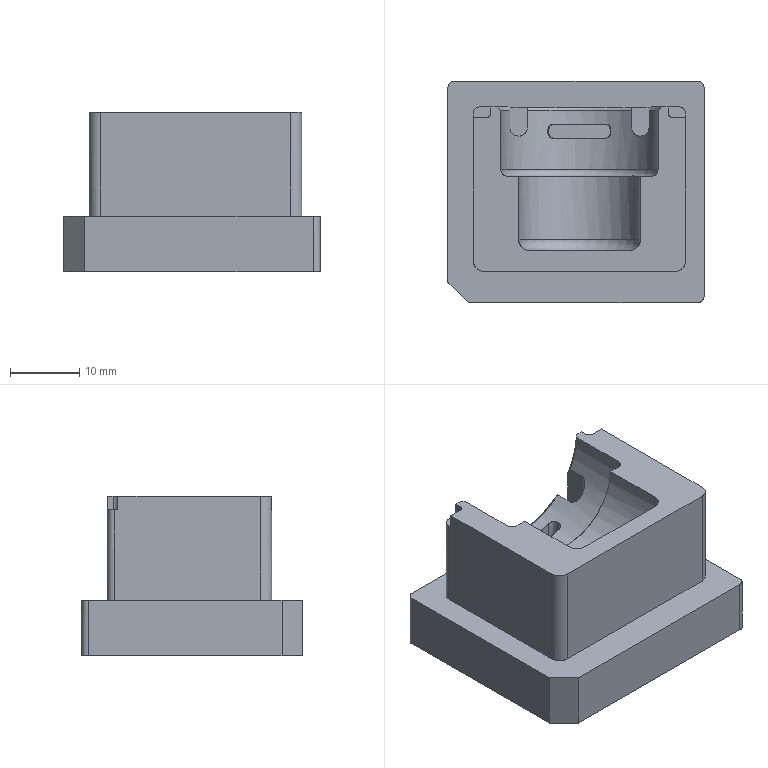NC program | PowerMill | posted with a generic post | part box 37 x 32 x 23 mm
Lines 1 to 1016 of 159067:
%
O0001
N104 ( POWERMILL CB  : 2026004.0)
N105 ( POST VER      : 2026.0.0.5161)
N106 ( OPTION FILE   : FANUC)
N107 ( OUTPUT WORKPLANE : WORLD)
N108 (  )
N109 ( TOOL LIST )
N110 (---------------------------------------)
N111 ( NO. | ID        | DIA.| TIP RAD|LENGTH)
N112 (---------------------------------------)
N113 (    1|D10C_2_1_1 |10.0 |  0.0   |78.44 )
N114 (   15|D3C_1_1    | 3.0 |  0.0   |66.32 )
N115 (   26|D1.5C_2_1  | 1.5 |  0.0   |68.34 )
N116 (    3|D10_1_1_1  |10.0 |  0.0   |78.16 )
N117 (   22|R1.5_2_1   | 3.0 |  1.5   |67.36 )
N118 (    6|R0.5_2_1   | 1.0 |  0.5   |66.36 )
N119 (   20|D1.5_2_1   | 1.5 |  0.0   |68.42 )
N120 (    8|D1_1_1     | 1.0 |  0.0   |57.32 )
N121 (   13|TEXT_D4_1_1| 4.0 |  0.3   |70.28 )
N122 (---------------------------------------)
N123 (  )
N124 ( NUMBER OF TOOLPATHS: 15.0 )
N125 ( ESTIMATED PROGRAM DURATION: 0 HOURS 22 MIN 2 SEC)
N126 (  )
N127 G00 G21 G80 G40 G17
N128 G90
N129 G54
N130 G53 Z0.0
N131 (---------------)
N132 ( START TOOLPATH : 粗公开粗01-扫面平行-D10C )
N133 (---------------)
N134 ( TOOL NO.    :1 )
N135 ( TOOL TYPE   : ENDMILL)
N136 ( TOOL ID     : D10C_2_1_1)
N137 ( TOOL DIA    : 10.0 LENGTH 78.44)
N138 T1
N139 M6
N140 S8000 M03
N141 G00 G90 X0.0 Y0.0
N142 G43 Z10.2 H1
N143
N144 G05 P10000 R4
N145 X26.15 Y18.65
N146 Z1.0
N147 G01 Z-0.2 F6000.0
N148 X21.15 F10000.0
N149 X-21.15
N150 Y13.3214
N151 X21.15
N152 Y7.9929
N153 X-21.15
N154 Y2.6643
N155 X21.15
N156 Y-2.6643
N157 X-21.15
N158 Y-7.9929
N159 X21.15
N160 Y-13.3214
N161 X-21.15
N162 Y-18.65
N163 X21.15
N164 X26.15
N165 G00 Z10.2
N166 G05 P0
N167 (---------------)
N168 ( END TOOLPATH : 粗公开粗01-扫面平行-D10C )
N169 (---------------)
N170 ( START TOOLPATH : 粗公开粗01-外形偏置-D10C )
N171 (---------------)
N172 G00 X0.4975 Y0.3775 Z9.8
N173 G05 P10000 R4
N174 X5.245 Y-24.424
N175 Z0.5648
N176 G01 Z-0.6352 F6000.0
N177 Y-23.8965 F10000.0
N178 G03 X0.4975 Y-19.149 I-4.7475 J0.0
N179 G01 X-21.509
N180 G02 X-22.509 Y-18.149 I0.0 J1.0
N181 G01 Y18.904
N182 G02 X-21.509 Y19.904 I1.0 J0.0
N183 G01 X22.504
N184 G02 X23.504 Y18.904 I0.0 J-1.0
N185 G01 Y-18.149
N186 G02 X22.504 Y-19.149 I-1.0 J0.0
N187 G01 X0.4975
N188 Y-16.65
N189 X-13.0375
N190 X-13.6116 Y-16.6379
N191 X-14.5843 Y-16.5183
N192 X-15.3577 Y-16.312
N193 X-16.1312 Y-16.0036
N194 X-16.9046 Y-15.5805
N195 X-17.5603 Y-15.091
N196 X-18.3552 Y-14.3176
N197 X-18.9402 Y-13.5442
N198 X-19.3631 Y-12.7708
N199 X-19.6712 Y-11.9973
N200 X-19.8772 Y-11.2239
N201 X-19.9796 Y-10.4505
N202 X-20.0085 Y-9.677
N203 Y10.432
N204 X-19.9983 Y11.0255
N205 X-19.8473 Y11.9789
N206 X-19.5822 Y12.7523
N207 X-19.2249 Y13.4316
N208 X-18.5428 Y14.2992
N209 X-17.678 Y15.0104
N210 X-16.9046 Y15.4268
N211 X-16.521 Y15.5751
N212 X-16.2887 Y15.6449
N213 X-16.169 Y15.6989
N214 X-16.0675 Y15.7821
N215 X-16.0077 Y15.846
N216 X-15.3577 Y16.4108
N217 X-15.0499 Y16.6195
N218 X-14.5843 Y16.8785
N219 X-13.8109 Y17.183
N220 X-13.0375 Y17.3538
N221 X-12.6625 Y17.3929
N222 X-11.4906 Y17.4045
N223 X-10.7172 Y17.3675
N224 X-9.9438 Y17.2129
N225 X-9.1703 Y16.9284
N226 X-8.5999 Y16.6195
N227 X-8.3969 Y16.4857
N228 X-7.6411 Y15.846
N229 X-6.893 Y15.0726
N230 X-6.3535 Y14.2992
N231 X-5.994 Y13.5258
N232 X-5.777 Y12.7523
N233 X-5.6845 Y11.9789
N234 X-5.6795 Y11.2055
N235 X-5.6794 Y10.6326
N236 X0.317 Y10.6393
N237 X0.3155 Y11.9856
N238 X0.3047 Y12.3391
N239 X0.2731 Y12.6914
N240 X0.1806 Y13.4648
N241 X0.1501 Y13.6851
N242 X0.1115 Y13.904
N243 X0.885
N244 X0.8467 Y13.6873
N245 X0.8164 Y13.4693
N246 X0.7233 Y12.6958
N247 X0.6913 Y12.341
N248 X0.6804 Y11.9849
N249 X0.6777 Y9.2986
N250 X0.4967 Y9.07
N251 X0.3185 Y9.293
N252 X0.317 Y10.6393
N253 X-5.6794 Y10.6326
N254 X-5.6789 Y6.9359
N255 G03 X-5.4485 Y6.5149 I0.5 J0.0001
N256 G01 X-5.3032 Y6.4218
N257 X-4.5638 Y5.7915
N258 X-3.9457 Y5.0181
N259 X-3.7563 Y4.7032
N260 X-3.5305 Y4.2446
N261 X-3.267 Y3.4712
N262 X-3.1329 Y2.6978
N263 X-3.1092 Y1.9244
N264 Y-2.8495
N265 G03 X-2.6093 Y-3.3495 I0.5 J0.0
N266 G01 X3.605 Y-3.35
N267 G03 X4.1051 Y-2.85 I0.0001 J0.5
N268 G01 X4.1049 Y1.9244
N269 X4.1284 Y2.6978
N270 X4.2633 Y3.4712
N271 X4.5264 Y4.2446
N272 X4.7513 Y4.7019
N273 X4.9416 Y5.0181
N274 X5.5248 Y5.7549
N275 X6.2982 Y6.4213
N276 X6.4442 Y6.5144
N277 G03 X6.6753 Y6.9359 I-0.2689 J0.4215
N278 G01 X6.6754 Y11.2055
N279 X6.6804 Y11.9789
N280 X6.7734 Y12.7523
N281 X6.9904 Y13.5258
N282 X7.3494 Y14.2992
N283 X7.8451 Y15.0196
N284 X8.6185 Y15.8273
N285 X9.3919 Y16.4852
N286 X9.5953 Y16.6195
N287 X10.1653 Y16.928
N288 X10.9388 Y17.2125
N289 X11.7122 Y17.3673
N290 X11.9831 Y17.3929
N291 X13.259 Y17.4045
N292 X14.0325 Y17.3539
N293 X14.8059 Y17.1833
N294 X15.5793 Y16.8789
N295 X16.0457 Y16.6195
N296 X16.3527 Y16.4115
N297 X17.0036 Y15.846
N298 X17.0643 Y15.781
N299 X17.1564 Y15.7035
N300 X17.2643 Y15.6502
N301 X17.8996 Y15.4272
N302 X18.5764 Y15.0726
N303 X19.4464 Y14.3912
N304 X20.1604 Y13.5258
N305 X20.5781 Y12.7523
N306 X20.8432 Y11.9789
N307 X20.9796 Y11.2055
N308 X21.0044 Y10.432
N309 Y-9.677
N310 X20.9933 Y-10.2384
N311 X20.8731 Y-11.2239
N312 X20.6671 Y-11.9973
N313 X20.359 Y-12.7708
N314 X19.936 Y-13.5442
N315 X19.4464 Y-14.2005
N316 X18.673 Y-14.9958
N317 X17.8996 Y-15.581
N318 X17.1262 Y-16.004
N319 X16.3527 Y-16.3122
N320 X15.5793 Y-16.5184
N321 X14.6075 Y-16.6379
N322 X14.0325 Y-16.65
N323 X0.4975
N324 Y-19.149
N325 G00 Z3.2296
N326 G01 X5.245 Y-24.424
N327 G00 Z0.1796
N328 G01 Z-1.0204 F6000.0
N329 Y-23.8965 F10000.0
N330 G03 X0.4975 Y-19.149 I-4.7475 J0.0
N331 G01 X-21.509
N332 G02 X-22.509 Y-18.149 I0.0 J1.0
N333 G01 Y18.904
N334 G02 X-21.509 Y19.904 I1.0 J0.0
N335 G01 X22.504
N336 G02 X23.504 Y18.904 I0.0 J-1.0
N337 G01 Y-18.149
N338 G02 X22.504 Y-19.149 I-1.0 J0.0
N339 G01 X0.4975
N340 Y-16.65
N341 X-13.0375
N342 X-13.6116 Y-16.6379
N343 X-14.5843 Y-16.5183
N344 X-15.3577 Y-16.312
N345 X-16.1312 Y-16.0036
N346 X-16.9046 Y-15.5805
N347 X-17.5603 Y-15.091
N348 X-18.3552 Y-14.3176
N349 X-18.9402 Y-13.5442
N350 X-19.3631 Y-12.7708
N351 X-19.6712 Y-11.9973
N352 X-19.8772 Y-11.2239
N353 X-19.9796 Y-10.4505
N354 X-20.0085 Y-9.677
N355 Y10.432
N356 X-19.9983 Y11.0256
N357 X-19.8474 Y11.9789
N358 X-19.5822 Y12.7523
N359 X-19.2249 Y13.4316
N360 X-18.5428 Y14.2992
N361 X-17.678 Y15.0104
N362 X-16.9046 Y15.4269
N363 X-16.5209 Y15.5751
N364 X-16.2887 Y15.6449
N365 X-16.169 Y15.6989
N366 X-16.0675 Y15.7822
N367 X-16.0077 Y15.846
N368 X-15.3577 Y16.4108
N369 X-15.0499 Y16.6195
N370 X-14.5843 Y16.8785
N371 X-13.8109 Y17.183
N372 X-13.0375 Y17.3538
N373 X-12.6625 Y17.3929
N374 X-11.4906 Y17.4045
N375 X-10.7172 Y17.3709
N376 X-9.9438 Y17.2217
N377 X-9.1703 Y16.9401
N378 X-8.6517 Y16.6475
N379 X-8.5999 Y16.6194
N380 X-8.5875 Y16.6112
N381 X-8.3969 Y16.5037
N382 X-7.6235 Y15.8538
N383 X-6.8666 Y15.0726
N384 X-6.3272 Y14.2992
N385 X-6.0766 Y13.7972
N386 X-5.967 Y13.5258
N387 X-5.75 Y12.7523
N388 X-5.6581 Y11.9789
N389 X-5.6531 Y11.2055
N390 X-5.653 Y10.5928
N391 X0.0935 Y10.5995
N392 X0.0919 Y11.9856
N393 X0.0816 Y12.3219
N394 X0.0518 Y12.6571
N395 X-0.0401 Y13.4305
N396 X-0.0952 Y13.7944
N397 X-0.1734 Y14.154
N398 X1.1706
N399 X1.0931 Y13.7988
N400 X1.0383 Y13.4394
N401 X0.9452 Y12.666
N402 X0.9145 Y12.3262
N403 X0.904 Y11.9852
N404 X0.901 Y9.214
N405 X0.4979 Y8.7094
N406 X0.0951 Y9.2135
N407 X0.0935 Y10.5995
N408 X-5.653 Y10.5928
N409 X-5.6523 Y6.9414
N410 G03 X-5.4192 Y6.5188 I0.5 J0.0001
N411 G01 X-5.3032 Y6.4455
N412 X-4.5308 Y5.7915
N413 X-3.9127 Y5.0181
N414 X-3.7563 Y4.763
N415 X-3.4975 Y4.2446
N416 X-3.2335 Y3.4712
N417 X-3.0999 Y2.6978
N418 X-3.0762 Y1.9244
N419 Y-2.8498
N420 G03 X-2.5909 Y-3.3496 I0.5 J0.0
N421 G01 X2.8684 Y-3.35
N422 X3.5715
N423 G03 X4.0715 Y-2.85 I0.0 J0.5
N424 G01 X4.0717 Y1.9244
N425 X4.0949 Y2.6978
N426 X4.2303 Y3.4712
N427 X4.4934 Y4.2446
N428 X4.7513 Y4.762
N429 X4.9085 Y5.0181
N430 X5.5248 Y5.7895
N431 X6.2982 Y6.4451
N432 X6.4147 Y6.5183
N433 G03 X6.6485 Y6.9416 I-0.2662 J0.4233
N434 G01 X6.649 Y11.2055
N435 X6.654 Y11.9789
N436 X6.7471 Y12.7523
N437 X6.964 Y13.5258
N438 X7.0716 Y13.795
N439 X7.323 Y14.2992
N440 X7.8451 Y15.0515
N441 X8.6117 Y15.846
N442 X9.3919 Y16.5033
N443 X9.5814 Y16.6102
N444 X9.5954 Y16.6194
N445 X9.6535 Y16.6509
N446 X10.1653 Y16.9397
N447 X10.9388 Y17.2215
N448 X11.7122 Y17.3708
N449 X11.9577 Y17.3929
N450 X13.259 Y17.4045
N451 X14.0325 Y17.354
N452 X14.8059 Y17.1833
N453 X15.5793 Y16.8789
N454 X16.0457 Y16.6195
N455 X16.3527 Y16.4115
N456 X17.0036 Y15.846
N457 X17.0642 Y15.781
N458 X17.1564 Y15.7035
N459 X17.2643 Y15.6502
N460 X17.8996 Y15.4272
N461 X18.5764 Y15.0726
N462 X19.4464 Y14.3913
N463 X20.1605 Y13.5258
N464 X20.5781 Y12.7523
N465 X20.8433 Y11.9789
N466 X20.9796 Y11.2055
N467 X21.0044 Y10.432
N468 Y-9.677
N469 X20.9933 Y-10.2384
N470 X20.8731 Y-11.2239
N471 X20.6671 Y-11.9973
N472 X20.359 Y-12.7708
N473 X19.936 Y-13.5442
N474 X19.4464 Y-14.2005
N475 X18.673 Y-14.9958
N476 X17.8996 Y-15.581
N477 X17.1262 Y-16.004
N478 X16.3527 Y-16.3122
N479 X15.5793 Y-16.5184
N480 X14.6075 Y-16.6379
N481 X14.0325 Y-16.65
N482 X0.4975
N483 Y-19.149
N484 G00 Z2.8444
N485 G01 X5.245 Y-24.424
N486 G00 Z-0.2056
N487 G01 Z-1.4056 F6000.0
N488 Y-23.8965 F10000.0
N489 G03 X0.4975 Y-19.149 I-4.7475 J0.0
N490 G01 X-21.509
N491 G02 X-22.509 Y-18.149 I0.0 J1.0
N492 G01 Y18.904
N493 G02 X-21.509 Y19.904 I1.0 J0.0
N494 G01 X22.504
N495 G02 X23.504 Y18.904 I0.0 J-1.0
N496 G01 Y-18.149
N497 G02 X22.504 Y-19.149 I-1.0 J0.0
N498 G01 X0.4975
N499 Y-16.65
N500 X-13.0375
N501 X-13.6116 Y-16.6379
N502 X-14.5843 Y-16.5183
N503 X-15.3577 Y-16.312
N504 X-16.1312 Y-16.0036
N505 X-16.9046 Y-15.5805
N506 X-17.5603 Y-15.091
N507 X-18.3552 Y-14.3176
N508 X-18.9402 Y-13.5442
N509 X-19.3631 Y-12.7708
N510 X-19.6712 Y-11.9973
N511 X-19.8772 Y-11.2239
N512 X-19.9796 Y-10.4505
N513 X-20.0085 Y-9.677
N514 Y10.432
N515 X-19.9983 Y11.0256
N516 X-19.8474 Y11.9789
N517 X-19.5823 Y12.7523
N518 X-19.2249 Y13.4317
N519 X-18.5428 Y14.2992
N520 X-17.678 Y15.0104
N521 X-16.9046 Y15.4269
N522 X-16.5209 Y15.5751
N523 X-16.2887 Y15.6449
N524 X-16.169 Y15.6989
N525 X-16.0674 Y15.7822
N526 X-16.0078 Y15.846
N527 X-15.3577 Y16.4108
N528 X-15.0499 Y16.6195
N529 X-14.5843 Y16.8785
N530 X-13.8109 Y17.183
N531 X-13.0375 Y17.3539
N532 X-13.0354 Y17.354
N533 X-12.6625 Y17.3928
N534 X-12.4026 Y17.3954
N535 X-12.264 Y17.4045
N536 X-11.9996 Y17.3994
N537 X-11.4906 Y17.4044
N538 X-10.8776 Y17.3778
N539 X-10.7172 Y17.3747
N540 X-9.9438 Y17.2309
N541 X-9.1703 Y16.957
N542 X-8.3969 Y16.5283
N543 X-7.6235 Y15.8911
N544 X-6.8298 Y15.0726
N545 X-6.2903 Y14.2992
N546 X-6.0766 Y13.8793
N547 X-5.9314 Y13.5258
N548 X-5.7144 Y12.7523
N549 X-5.6213 Y11.9789
N550 X-5.6167 Y11.2055
N551 X-5.6179 Y6.9538
N552 G03 X-5.3811 Y6.5285 I0.5 J-0.0002
N553 G01 X-5.3032 Y6.4803
N554 X-4.5298 Y5.8438
N555 X-3.861 Y5.0181
N556 X-3.4449 Y4.2446
N557 X-3.182 Y3.4712
N558 X-3.0481 Y2.6978
N559 X-3.025 Y1.9244
N560 Y-2.8489
N561 G03 X-2.5251 Y-3.3489 I0.5 J0.0
N562 G01 X3.5205 Y-3.3499
N563 G03 X4.0206 Y-2.8499 I0.0001 J0.5
N564 G01 X4.0208 Y1.9244
N565 X4.044 Y2.6978
N566 X4.1783 Y3.4712
N567 X4.4413 Y4.2446
N568 X4.8565 Y5.0181
N569 X5.474 Y5.7915
N570 X6.2982 Y6.4798
N571 X6.3754 Y6.5276
N572 G03 X6.6123 Y6.9529 I-0.2631 J0.4251
N573 G01 X6.6112 Y11.0997
N574 X1.4938 Y11.3269
N575 X1.4338 Y9.9765
N576 G02 X-0.4482 Y9.975 I-0.9411 J0.0365
N577 G01 X-0.5211 Y11.6968
N578 X-0.6211 Y13.3605
N579 G02 X0.2541 Y14.2839 I0.8696 J0.0523
N580 G01 X0.7548 Y14.2807
N581 G02 X1.6185 Y13.3517 I-0.0056 J-0.8712
N582 G01 X1.5138 Y11.7771
N583 X1.4938 Y11.3269
N584 X6.6112 Y11.0997
N585 Y11.2055
N586 X6.6161 Y11.9789
N587 X6.7091 Y12.7523
N588 X6.9264 Y13.5258
N589 X7.0716 Y13.8792
N590 X7.2849 Y14.2992
N591 X7.8243 Y15.0726
N592 X8.6185 Y15.8902
N593 X9.3919 Y16.5277
N594 X10.1653 Y16.9566
N595 X10.9388 Y17.2307
N596 X11.7122 Y17.3746
N597 X11.767 Y17.3757
N598 X11.9577 Y17.3928
N599 X13.2539 Y17.4044
N600 X13.259 Y17.4045
N601 X14.0325 Y17.354
N602 X14.8059 Y17.1833
N603 X15.5793 Y16.8789
N604 X16.0457 Y16.6195
N605 X16.3527 Y16.4115
N606 X17.0037 Y15.846
N607 X17.0642 Y15.781
N608 X17.1564 Y15.7035
N609 X17.2644 Y15.6502
N610 X17.8996 Y15.4272
N611 X18.5765 Y15.0726
N612 X19.4464 Y14.3913
N613 X20.1605 Y13.5258
N614 X20.5782 Y12.7523
N615 X20.8433 Y11.9789
N616 X20.9797 Y11.2055
N617 X21.0044 Y10.432
N618 Y-9.677
N619 X20.9933 Y-10.2384
N620 X20.8731 Y-11.2239
N621 X20.6671 Y-11.9973
N622 X20.359 Y-12.7708
N623 X19.936 Y-13.5442
N624 X19.4464 Y-14.2005
N625 X18.673 Y-14.9958
N626 X17.8996 Y-15.581
N627 X17.1262 Y-16.004
N628 X16.3527 Y-16.3122
N629 X15.5793 Y-16.5184
N630 X14.6075 Y-16.6379
N631 X14.0325 Y-16.65
N632 X0.4975
N633 Y-19.149
N634 G00 Z2.4592
N635 G01 X5.245 Y-24.424
N636 G00 Z-0.5908
N637 G01 Z-1.7908 F6000.0
N638 Y-23.8965 F10000.0
N639 G03 X0.4975 Y-19.149 I-4.7475 J0.0
N640 G01 X-21.509
N641 G02 X-22.509 Y-18.149 I0.0 J1.0
N642 G01 Y18.904
N643 G02 X-21.509 Y19.904 I1.0 J0.0
N644 G01 X22.504
N645 G02 X23.504 Y18.904 I0.0 J-1.0
N646 G01 Y-18.149
N647 G02 X22.504 Y-19.149 I-1.0 J0.0
N648 G01 X0.4975
N649 Y-16.65
N650 X-13.0375
N651 X-13.6116 Y-16.6379
N652 X-14.5843 Y-16.5183
N653 X-15.3577 Y-16.312
N654 X-16.1312 Y-16.0036
N655 X-16.9046 Y-15.5805
N656 X-17.5603 Y-15.091
N657 X-18.3552 Y-14.3176
N658 X-18.9402 Y-13.5442
N659 X-19.3631 Y-12.7708
N660 X-19.6712 Y-11.9973
N661 X-19.8772 Y-11.2239
N662 X-19.9796 Y-10.4505
N663 X-20.0085 Y-9.677
N664 Y10.432
N665 X-19.9983 Y11.0256
N666 X-19.8474 Y11.9789
N667 X-19.5823 Y12.7523
N668 X-19.2249 Y13.4317
N669 X-18.5428 Y14.2992
N670 X-17.678 Y15.0104
N671 X-16.9046 Y15.4269
N672 X-16.5209 Y15.5751
N673 X-16.2887 Y15.6449
N674 X-16.169 Y15.6989
N675 X-16.0674 Y15.7823
N676 X-16.0078 Y15.846
N677 X-15.3577 Y16.4108
N678 X-15.0499 Y16.6195
N679 X-14.5843 Y16.8785
N680 X-13.8109 Y17.183
N681 X-13.0375 Y17.3539
N682 X-12.6625 Y17.3929
N683 X-12.6524
N684 X-12.4026 Y17.3954
N685 X-12.264 Y17.4044
N686 X-11.9996 Y17.3993
N687 X-11.4906 Y17.4044
N688 X-11.2261 Y17.3929
N689 X-10.867
N690 X-10.7568 Y17.3754
N691 X-10.7172 Y17.3747
N692 X-10.5164 Y17.3373
N693 X-9.9438 Y17.2466
N694 X-9.1703 Y16.9825
N695 X-8.4794 Y16.6195
N696 X-7.6235 Y15.9469
N697 X-6.8501 Y15.167
N698 X-6.228 Y14.2992
N699 X-6.0766 Y14.0113
N700 X-5.8691 Y13.5258
N701 X-5.6521 Y12.7523
N702 X-5.559 Y11.9789
N703 X-5.5542 Y11.2055
N704 X-5.5537 Y6.9636
N705 G03 X-5.315 Y6.5374 I0.5 J0.0001
N706 G01 X-5.3032 Y6.5302
N707 X-4.5298 Y5.9188
N708 X-4.4016 Y5.7915
N709 X-3.783 Y5.0181
N710 X-3.3684 Y4.2446
N711 X-3.1052 Y3.4712
N712 X-2.9829 Y2.81
N713 X-2.947 Y1.9244
N714 Y-2.8494
N715 G03 X-2.4679 Y-3.3489 I0.5 J0.0
N716 G01 X3.4424 Y-3.35
N717 G03 X3.942 Y-2.85 I-0.0004 J0.5
N718 G01 X3.9423 Y1.9244
N719 X3.9663 Y2.6978
N720 X4.1011 Y3.4712
N721 X4.3642 Y4.2446
N722 X4.7513 Y4.9744
N723 X5.3966 Y5.7915
N724 X5.5248 Y5.9172
N725 X6.3526 Y6.5649
N726 G03 X6.5498 Y6.9629 I-0.3028 J0.3979
N727 G01 X6.549 Y11.2055
N728 X6.5535 Y11.8606
N729 X1.5211 Y12.4313
N730 X1.4606 Y11.8982
N731 X1.3667 Y10.0008
N732 G02 X-0.3737 Y9.9978 I-0.8703 J0.0402
N733 G01 X-0.4782 Y11.9801
N734 X-0.573 Y12.8902
N735 X-0.6296 Y13.3197
N736 G02 X0.2138 Y14.2742 I0.8371 J0.1102
N737 G01 X0.7945 Y14.2698
N738 G02 X1.6218 Y13.3197 I-0.0063 J-0.8408
N739 G01 X1.5211 Y12.4313
N740 X6.5535 Y11.8606
N741 X6.5543 Y11.9789
N742 X6.6473 Y12.7523
N743 X6.8649 Y13.5258
N744 X7.0716 Y14.0099
N745 X7.2232 Y14.2992
N746 X7.7626 Y15.0726
N747 X8.6185 Y15.946
N748 X9.3919 Y16.5658
N749 X10.1653 Y16.9822
N750 X10.9388 Y17.2464
N751 X11.7122 Y17.3805
N752 X11.8432 Y17.3825
N753 X11.9577 Y17.3928
N754 X13.2431 Y17.4042
N755 X13.259 Y17.4045
N756 X14.0325 Y17.354
N757 X14.8059 Y17.1833
N758 X15.5793 Y16.8789
N759 X16.0458 Y16.6195
N760 X16.3527 Y16.4115
N761 X17.0037 Y15.846
N762 X17.0642 Y15.7811
N763 X17.1564 Y15.7035
N764 X17.2644 Y15.6502
N765 X17.8996 Y15.4273
N766 X18.5765 Y15.0726
N767 X19.4464 Y14.3913
N768 X20.1605 Y13.5258
N769 X20.5782 Y12.7523
N770 X20.8433 Y11.9789
N771 X20.9797 Y11.2055
N772 X21.0044 Y10.432
N773 Y-9.677
N774 X20.9933 Y-10.2384
N775 X20.8731 Y-11.2239
N776 X20.6671 Y-11.9973
N777 X20.359 Y-12.7708
N778 X19.936 Y-13.5442
N779 X19.4464 Y-14.2005
N780 X18.673 Y-14.9958
N781 X17.8996 Y-15.581
N782 X17.1262 Y-16.004
N783 X16.3527 Y-16.3122
N784 X15.5793 Y-16.5184
N785 X14.6075 Y-16.6379
N786 X14.0325 Y-16.65
N787 X0.4975
N788 Y-19.149
N789 G00 Z2.074
N790 G01 X5.245 Y-24.424
N791 G00 Z-0.976
N792 G01 Z-2.176 F6000.0
N793 Y-23.8965 F10000.0
N794 G03 X0.4975 Y-19.149 I-4.7475 J0.0
N795 G01 X-21.509
N796 G02 X-22.509 Y-18.149 I0.0 J1.0
N797 G01 Y18.904
N798 G02 X-21.509 Y19.904 I1.0 J0.0
N799 G01 X22.504
N800 G02 X23.504 Y18.904 I0.0 J-1.0
N801 G01 Y-18.149
N802 G02 X22.504 Y-19.149 I-1.0 J0.0
N803 G01 X0.4975
N804 Y-16.65
N805 X-13.0375
N806 X-13.6116 Y-16.6379
N807 X-14.5843 Y-16.5183
N808 X-15.3577 Y-16.312
N809 X-16.1312 Y-16.0036
N810 X-16.9046 Y-15.5805
N811 X-17.5603 Y-15.091
N812 X-18.3552 Y-14.3176
N813 X-18.9402 Y-13.5442
N814 X-19.3631 Y-12.7708
N815 X-19.6712 Y-11.9973
N816 X-19.8772 Y-11.2239
N817 X-19.9796 Y-10.4505
N818 X-20.0085 Y-9.677
N819 Y10.432
N820 X-19.9983 Y11.0257
N821 X-19.8475 Y11.9789
N822 X-19.5823 Y12.7523
N823 X-19.2249 Y13.4317
N824 X-18.5429 Y14.2992
N825 X-17.678 Y15.0104
N826 X-16.9046 Y15.427
N827 X-16.5209 Y15.5751
N828 X-16.2887 Y15.6449
N829 X-16.1689 Y15.6989
N830 X-16.0674 Y15.7823
N831 X-16.0078 Y15.846
N832 X-15.3577 Y16.4109
N833 X-15.0499 Y16.6195
N834 X-14.5843 Y16.8785
N835 X-13.8109 Y17.1831
N836 X-13.0375 Y17.3539
N837 X-12.6626 Y17.3929
N838 X-12.6473
N839 X-12.4026 Y17.3953
N840 X-12.264 Y17.4044
N841 X-11.9996 Y17.3993
N842 X-11.4906 Y17.4043
N843 X-11.2273 Y17.3929
N844 X-10.8056
N845 X-9.9438 Y17.2623
N846 X-9.1703 Y17.0081
N847 X-8.3969 Y16.6062
N848 X-7.6235 Y16.0052
N849 X-6.7052 Y15.0726
N850 X-6.1657 Y14.2992
N851 X-5.8068 Y13.5258
N852 X-5.5898 Y12.7523
N853 X-5.4967 Y11.9789
N854 X-5.4918 Y11.2055
N855 X-5.4901 Y6.9772
N856 G03 X-5.2728 Y6.5649 I0.5 J0.0002
N857 G01 X-4.5298 Y5.997
N858 X-4.3177 Y5.7915
N859 X-3.7563 Y5.1016
N860 X-3.2843 Y4.2446
N861 X-3.0211 Y3.4712
N862 X-2.8867 Y2.6978
N863 X-2.869 Y1.9244
N864 Y-2.8492
N865 G03 X-2.3822 Y-3.349 I0.5 J0.0
N866 G01 X1.9966 Y-3.3498
N867 X3.3641 Y-3.3499
N868 G03 X3.8641 Y-2.8499 I0.0 J0.5
N869 G01 X3.8639 Y1.9244
N870 X3.8827 Y2.6978
N871 X3.9779 Y3.3004
N872 X4.2805 Y4.2446
N873 X4.6956 Y5.0181
N874 X5.3136 Y5.7915
N875 X5.5248 Y5.9966
N876 X6.2886 Y6.5756
N877 G03 X6.4865 Y6.974 I-0.3021 J0.3984
N878 G01 X6.4868 Y11.2055
N879 X6.4925 Y11.9789
N880 X6.5336 Y12.3208
N881 X1.0884 Y13.0216
N882 G02 X-0.109 Y13.0316 I-0.5981 J0.0769
N883 G01 X-0.1634 Y13.5187
N884 G02 X0.3158 Y14.0507 I0.4759 J0.0532
N885 G01 X0.6794 Y14.0482
N886 G02 X1.1511 Y13.5083 I-0.0033 J-0.4788
N887 G01 X1.0884 Y13.0216
N888 X6.5336 Y12.3208
N889 X6.5855 Y12.7523
N890 X6.8019 Y13.5258
N891 X7.1615 Y14.2992
N892 X7.7009 Y15.0726
N893 X8.6185 Y16.0043
N894 X9.3919 Y16.6057
N895 X10.1653 Y17.0078
N896 X10.9388 Y17.2621
N897 X11.7122 Y17.3863
N898 X11.9124 Y17.3887
N899 X11.9577 Y17.3927
N900 X13.2036 Y17.4038
N901 X13.259 Y17.4045
N902 X14.0325 Y17.354
N903 X14.8059 Y17.1834
N904 X15.5793 Y16.8789
N905 X16.0458 Y16.6195
N906 X16.3527 Y16.4116
N907 X17.0037 Y15.846
N908 X17.0642 Y15.7811
N909 X17.1564 Y15.7035
N910 X17.2644 Y15.6502
N911 X17.8996 Y15.4273
N912 X18.5765 Y15.0726
N913 X19.4464 Y14.3913
N914 X20.1605 Y13.5258
N915 X20.5782 Y12.7523
N916 X20.8433 Y11.9789
N917 X20.9797 Y11.2055
N918 X21.0044 Y10.432
N919 Y-9.677
N920 X20.9933 Y-10.2384
N921 X20.8731 Y-11.2239
N922 X20.6671 Y-11.9973
N923 X20.359 Y-12.7708
N924 X19.936 Y-13.5442
N925 X19.4464 Y-14.2005
N926 X18.673 Y-14.9958
N927 X17.8996 Y-15.581
N928 X17.1262 Y-16.004
N929 X16.3527 Y-16.3123
N930 X15.5793 Y-16.5185
N931 X14.6075 Y-16.6379
N932 X14.0325 Y-16.65
N933 X0.4975
N934 Y-19.149
N935 G00 Z1.6839
N936 G01 X5.245 Y-24.424
N937 G00 Z-1.3661
N938 G01 Z-2.5661 F6000.0
N939 Y-23.8965 F10000.0
N940 G03 X0.4975 Y-19.149 I-4.7475 J0.0
N941 G01 X-21.509
N942 G02 X-22.509 Y-18.149 I0.0 J1.0
N943 G01 Y18.904
N944 G02 X-21.509 Y19.904 I1.0 J0.0
N945 G01 X22.504
N946 G02 X23.504 Y18.904 I0.0 J-1.0
N947 G01 Y-18.149
N948 G02 X22.504 Y-19.149 I-1.0 J0.0
N949 G01 X0.4975
N950 Y-16.65
N951 X-13.0375
N952 X-13.6116 Y-16.6379
N953 X-14.5843 Y-16.5183
N954 X-15.3577 Y-16.312
N955 X-16.1312 Y-16.0036
N956 X-16.9046 Y-15.5805
N957 X-17.5603 Y-15.091
N958 X-18.3552 Y-14.3176
N959 X-18.9402 Y-13.5442
N960 X-19.3631 Y-12.7708
N961 X-19.6712 Y-11.9973
N962 X-19.8772 Y-11.2239
N963 X-19.9796 Y-10.4505
N964 X-20.0085 Y-9.677
N965 Y11.2055
N966 X-19.9581 Y11.9789
N967 X-19.8233 Y12.7523
N968 X-19.5711 Y13.5258
N969 X-19.2249 Y14.2586
N970 X-18.6785 Y15.0726
N971 X-18.4514 Y15.3414
N972 X-17.947 Y15.846
N973 X-17.678 Y16.0733
N974 X-16.9046 Y16.5971
N975 X-16.1312 Y16.9665
N976 X-15.3577 Y17.2189
N977 X-14.5843 Y17.3539
N978 X-14.2043 Y17.3929
N979 X-12.6422
N980 X-12.4026 Y17.3953
N981 X-12.264 Y17.4043
N982 X-11.9996 Y17.3992
N983 X-11.4906 Y17.4043
N984 X-11.2284 Y17.3929
N985 X-10.7254
N986 X-9.9438 Y17.28
N987 X-9.1703 Y17.0422
N988 X-8.3969 Y16.6564
N989 X-7.6235 Y16.0808
N990 X-6.8501 Y15.3271
N991 X-6.6195 Y15.0726
N992 X-6.0801 Y14.2992
N993 X-5.7211 Y13.5258
N994 X-5.5034 Y12.7523
N995 X-5.4111 Y11.9789
N996 X-5.4061 Y11.2055
N997 X-5.4089 Y6.9982
N998 G03 X-5.1641 Y6.5678 I0.5 J-0.0004
N999 G01 X-5.1592 Y6.5649
N1000 X-4.5298 Y6.098
N1001 X-4.204 Y5.7915
N1002 X-3.7563 Y5.2623
N1003 X-3.586 Y5.0181
N1004 X-3.1708 Y4.2446
N1005 X-2.9077 Y3.4712
N1006 X-2.7729 Y2.6978
N1007 X-2.7495 Y1.9244
N1008 Y-2.8491
N1009 G03 X-2.2545 Y-3.3491 I0.5 J0.0
N1010 G01 X-1.0928 Y-3.3493
N1011 X3.2449 Y-3.3499
N1012 G03 X3.745 Y-2.85 I0.0001 J0.5
N1013 G01 X3.7452 Y1.9244
N1014 X3.769 Y2.6978
N1015 X3.9036 Y3.4712
N1016 X4.1666 Y4.2446
N1017 X4.5818 Y5.0181
N1018 X4.7513 Y5.2614
N1019 X5.1999 Y5.7915
N1020 X5.5248 Y6.0972
N1021 X6.155 Y6.5649
N1022 X6.1564 Y6.5657
N1023 G03 X6.4023 Y6.9964 I-0.2541 J0.4306
N1024 G01 X6.402 Y10.6474
N1025 X0.6557 Y10.6528
N1026 X0.6545 Y9.3213
N1027 X0.4979 Y9.1363
N1028 X0.3401 Y9.3229
N1029 X0.3389 Y11.9813
N1030 X0.3287 Y12.3214
N1031 X0.2984 Y12.6603
N1032 X0.2061 Y13.4337
N1033 X0.1511 Y13.796
N1034 X0.0732 Y14.154
N1035 X0.9231
N1036 X0.8455 Y13.7975
N1037 X0.7906 Y13.4368
N1038 X0.6978 Y12.6634
N1039 X0.6673 Y12.3244
N1040 X0.6569 Y11.9842
N1041 X0.6557 Y10.6528
N1042 X6.402 Y10.6474
N1043 X6.4019 Y11.2055
N1044 X6.4069 Y11.9789
N1045 X6.4997 Y12.7523
N1046 X6.717 Y13.5258
N1047 X7.0716 Y14.291
N1048 X7.6153 Y15.0726
N1049 X7.8451 Y15.3262
N1050 X8.6185 Y16.0794
N1051 X9.3336 Y16.6195
N1052 X10.1653 Y17.0419
N1053 X10.9388 Y17.2798
N1054 X11.7122 Y17.3921
N1055 X12.0457 Y17.3935
N1056 X13.2036 Y17.4038
N1057 X13.259 Y17.4044
N1058 X13.3475 Y17.3987
N1059 X14.8059 Y17.4045
N1060 X15.5793 Y17.3541
N1061 X16.3527 Y17.2192
N1062 X17.1262 Y16.9669
N1063 X17.861 Y16.6195
N1064 X18.673 Y16.074
N1065 X18.9429 Y15.846
N1066 X19.4464 Y15.3424
N1067 X19.6743 Y15.0726
N1068 X20.1978 Y14.2992
N1069 X20.567 Y13.5258
N1070 X20.8192 Y12.7523
N1071 X20.954 Y11.9789
N1072 X21.0044 Y11.2055
N1073 Y-9.677
N1074 X20.9933 Y-10.2384
N1075 X20.8731 Y-11.2239
N1076 X20.6671 Y-11.9973
N1077 X20.359 Y-12.7708
N1078 X19.936 Y-13.5442
N1079 X19.4464 Y-14.2005
N1080 X18.673 Y-14.9958
N1081 X17.8996 Y-15.581
N1082 X17.1262 Y-16.004
N1083 X16.3527 Y-16.3123
N1084 X15.5793 Y-16.5185
N1085 X14.6075 Y-16.6379
N1086 X14.0325 Y-16.65
N1087 X0.4975
N1088 Y-19.149
N1089 G00 Z1.2938
N1090 G01 X5.245 Y-24.424
N1091 G00 Z-1.7562
N1092 G01 Z-2.9562 F6000.0
N1093 Y-23.8965 F10000.0
N1094 G03 X0.4975 Y-19.149 I-4.7475 J0.0
N1095 G01 X-21.509
N1096 G02 X-22.509 Y-18.149 I0.0 J1.0
N1097 G01 Y18.904
N1098 G02 X-21.509 Y19.904 I1.0 J0.0
N1099 G01 X22.504
N1100 G02 X23.504 Y18.904 I0.0 J-1.0
N1101 G01 Y-18.149
N1102 G02 X22.504 Y-19.149 I-1.0 J0.0
N1103 G01 X0.4975
N1104 Y-16.65
N1105 X-13.0375
N1106 X-13.6116 Y-16.6379
N1107 X-14.5843 Y-16.5183
N1108 X-15.3577 Y-16.312
N1109 X-16.1312 Y-16.0036
N1110 X-16.9046 Y-15.5805
N1111 X-17.5603 Y-15.091
N1112 X-18.3552 Y-14.3176
N1113 X-18.9402 Y-13.5442